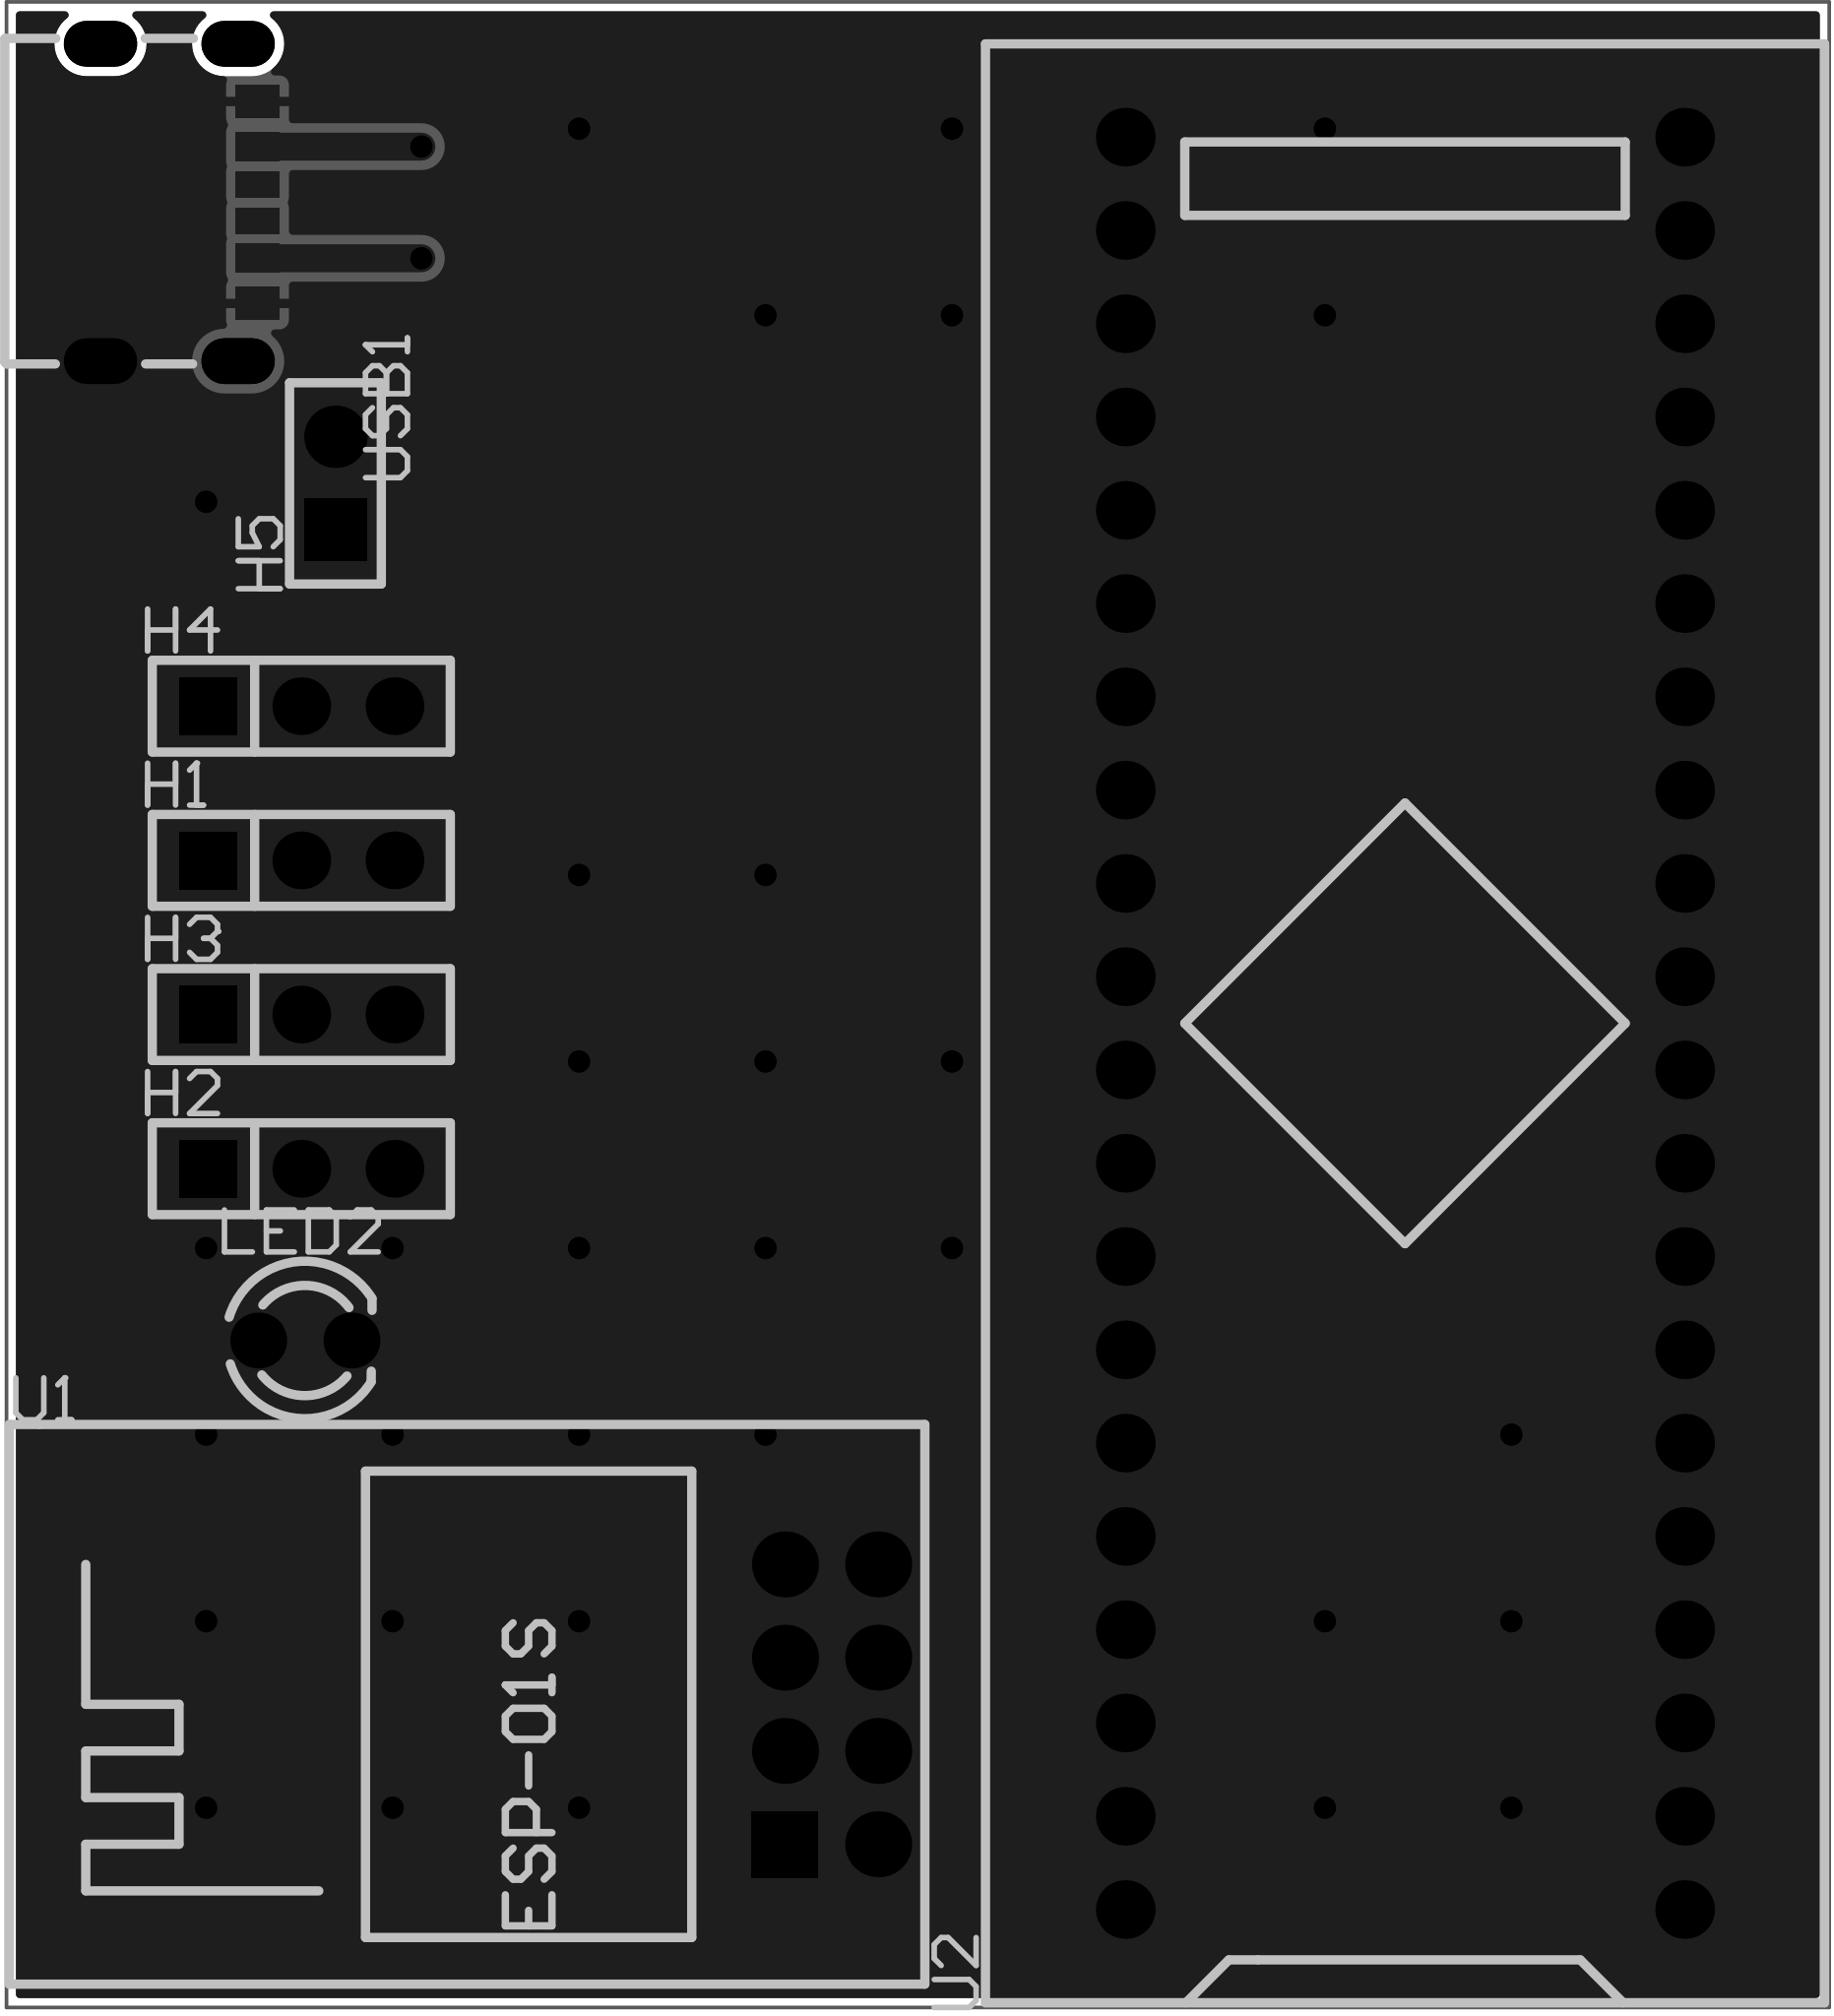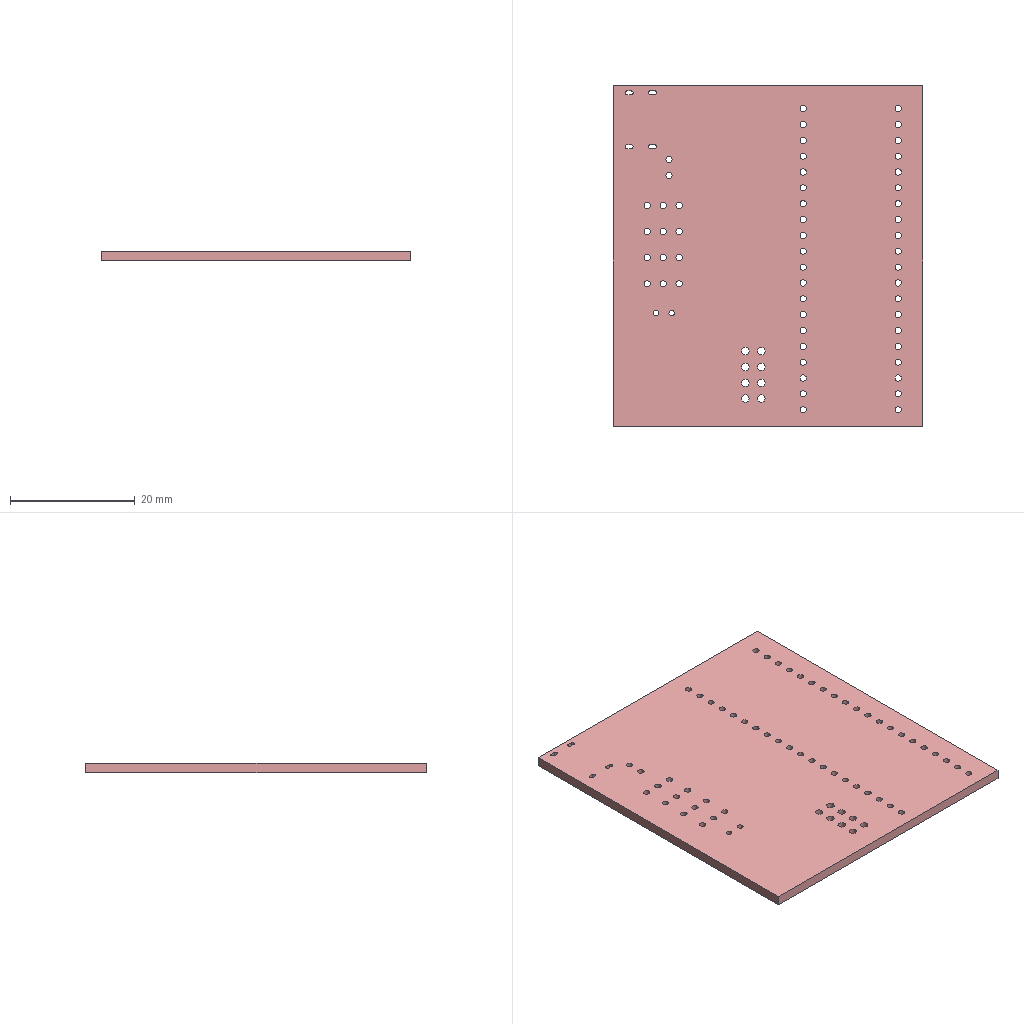Circuit board layout | Altium Designer | box 49.7 x 54.6 x 1.6 mm
Layer stack:
# Altium Designer layer stack of  (unit mm; dielectric type: 0 none, 1 core, 2 prepreg, 3 surface material)
index,name,kind,layer,copper_thickness_mm,dielectric_type,dielectric_thickness_mm,dielectric_material,dielectric_constant
0,Top Paste Mask Layer,other,,,,,,
1,Top Silkscreen Layer,other,,,,,,
2,Top Solder Mask Layer,dielectric,,,3,0.01,,3.3
3,Top Layer,copper,Top Layer,0.035,,,,
4,Dielectric1,dielectric,,,3,1.51,FR4,4.5
5,Bottom Layer,copper,Bottom Layer,0.035,,,,
6,Bottom Solder Mask Layer,dielectric,,,3,0.01,,3.3
7,Bottom Silkscreen Layer,other,,,,,,
8,Bottom Paste Mask Layer,other,,,,,,
# drill layer pairs: low layer,high layer
drill_pair,Top Layer,Bottom Layer
Part placement:
Designator,Comment,Layer,Footprint,Center-X(mm),Center-Y(mm),Rotation
H1,,TopLayer,HDR-TH_3P-P2.54-V-F,89.692,108.959,0
H2,,TopLayer,HDR-TH_3P-P2.54-V-F,89.692,100.562,0
H3,,TopLayer,HDR-TH_3P-P2.54-V-F,89.692,104.76,0
H4,,TopLayer,HDR-TH_3P-P2.54-V-F,89.692,113.157,0
U1,ESP-01S,TopLayer,WIFIM-TH_ESP-01S,104.14,85.979,90
U2,STM32F103C8T6最小系统开发板,TopLayer,CONN-TH_L53.3-W22.9_STM32F103C8T6-CARD,119.761,104.521,90
LED2,,TopLayer,LED_TH-3mm,89.789,95.885,0
USB1,,TopLayer,USB__TYPE-C-6P,86.36,126.873,270
H5,,TopLayer,HDR-TH_2P-P2.54-V-F,90.621,119.224,90
Pad and via stacks:
# Altium Designer via and pad stacks of  (unit mm). Each distinct definition once, with the count of objects using it.
# via: kind,start_layer,end_layer,hole_mm,diameter_mm,mode(0 simple;1 top-mid-bottom;2 full stack),diameter_per_layer,count,example_net
# pad: kind,layer,hole_mm,hole_type(0 round;1 square;2 slot),plating,top_size,top_shape(1 round;2 rect;3 octagon;9 rounded rect),mid_size,bottom_size,mode,footprint,size_per_layer,count,example
pad,Multi-Layer,1.02,0,plated,1.575x1.575,1,1.575x1.575,1.575x1.575,0,HDR-TH_3P-P2.54-V-F,,8,H1.3
pad,Multi-Layer,1.02,0,plated,1.575x1.575,2,1.575x1.575,1.575x1.575,0,HDR-TH_3P-P2.54-V-F,,4,H1.1
pad,Multi-Layer,1.2,0,plated,1.8x1.8,2,1.8x1.8,1.8x1.8,0,WIFIM-TH_ESP-01S,,1,U1.1
pad,Multi-Layer,1.2,0,plated,1.8x1.8,1,1.8x1.8,1.8x1.8,0,WIFIM-TH_ESP-01S,,7,U1.2
pad,Multi-Layer,1,0,plated,1.6x1.6,1,1.6x1.6,1.6x1.6,0,CONN-TH_L53.3-W22.9_STM32F103C8T6-CARD,,40,U2.1
pad,Multi-Layer,0.9144,0,plated,1.524x1.524,1,1.524x1.524,1.524x1.524,0,LED_TH-3mm,,2,LED2.1
pad,Multi-Layer,0.6,2,plated,1.25x2,1,1.25x2,1.25x2,0,USB_ TYPE-C-6P,,4,USB1.8
pad,Multi-Layer,1,0,plated,1.7x1.7,2,1.7x1.7,1.7x1.7,0,HDR-TH_2P-P2.54-V-F,,1,H5.1
pad,Multi-Layer,1,0,plated,1.7x1.7,1,1.7x1.7,1.7x1.7,0,HDR-TH_2P-P2.54-V-F,,1,H5.2
pad,Top Layer,0,0,plated,0.7x1.2,2,0.7x1.2,0.7x1.2,0,USB_ TYPE-C-6P,,2,USB1.A5
pad,Top Layer,0,0,plated,0.8x1.2,2,0.8x1.2,0.8x1.2,0,USB_ TYPE-C-6P,,2,USB1.B9
pad,Top Layer,0,0,plated,0.9x1.2,2,0.9x1.2,0.9x1.2,0,USB_ TYPE-C-6P,,2,USB1.B12
via,Top Layer,Bottom Layer,0.3048,0.61,0,,34,GND
Copper pours:
name,layer,net,type(0 solid;1 hatched;2 none)
Bottom Layer-GND,Bottom Layer,GND,0
Top Layer-GND,Top Layer,GND,0